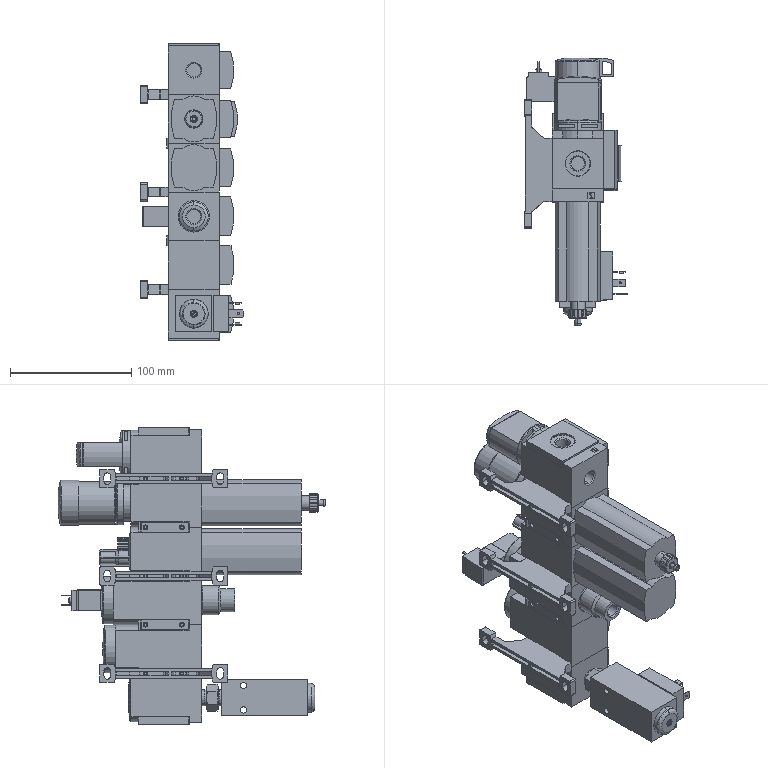Part | STEP file | 542315 MSB4-1_4_C3J4M1D1A1F3-WP_5 | 22 solids | 2755 faces | box 85 x 221.2 x 244.7 mm | volume 1168039 mm3 | plane 1702 | cylinder 757 | cone 252 | spline 44 | commonest cylinder face diameters 1 x129 2 x47 3 x46 3.8 x38 11.445 x34 1.6 x33